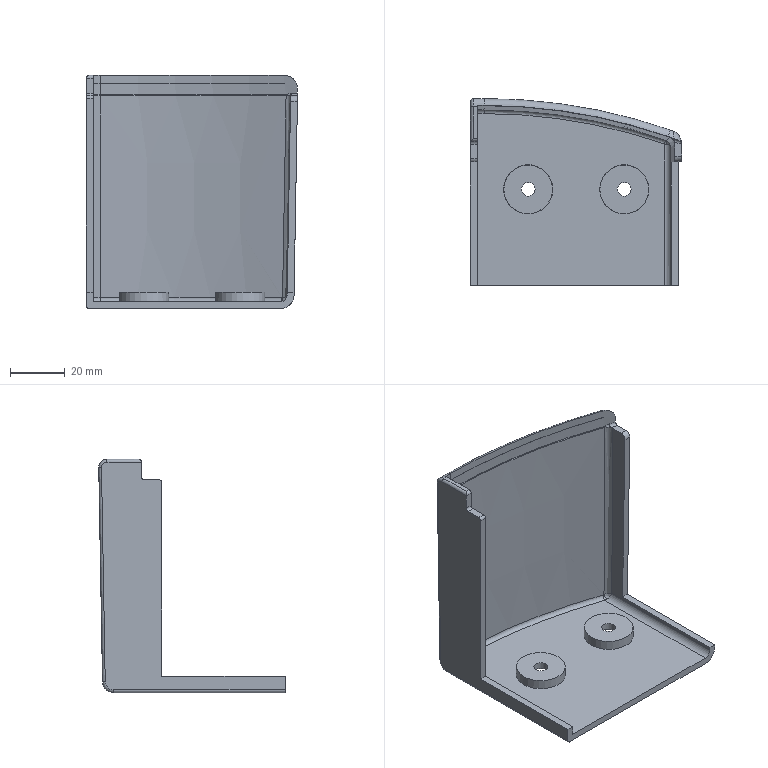Part | STEP file | HGR | 1 solid | 67 faces | box 76.869 x 67.947 x 85 mm | volume 33917 mm3 | plane 23 | cylinder 17 | spline 11 | torus 10 | cone 6 | commonest cylinder face diameters 2 x6 5 x3 10 x2 1 x1 3 x1 4 x1